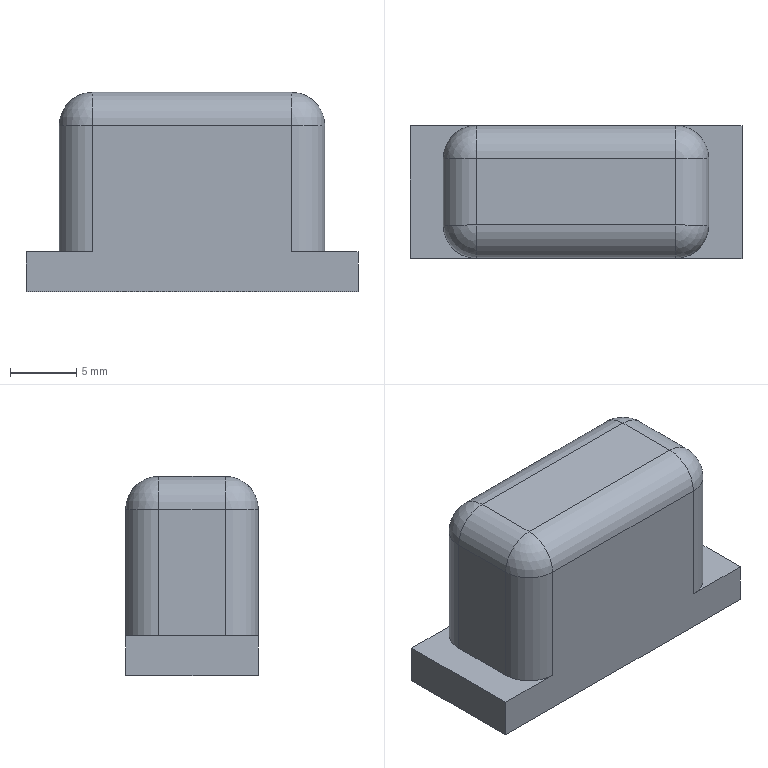NC program | NX | posted with a generic post | part box 25 x 10 x 15 mm
Whole program:
N10 G17 G21 G94 G90
(FLOOR_WALL_COPY , TOOL : D50)
N12 T01 M6
N14 G54
N16 G17 G0 G90 X-42.5 Y0. S4000 M3
N18 G43 Z30. H1
N20 Z5.666
N22 G94 G1 Z2.666 F1000.
N24 X-39.5
N26 X39.5
N28 X42.5
N30 Z5.666
N32 G0 Z30.
N34 X-42.5
N36 Z5.333
N38 G1 Z2.333
N40 X-39.5
N42 X39.5
N44 X42.5
N46 Z5.333
N48 G0 Z30.
N50 X-42.5
N52 Z5.
N54 G1 Z2.
N56 X-39.5
N58 X39.5
N60 X42.5
N62 Z5.
N64 G0 Z30.
N66 X-42.5
N68 Z4.667
N70 G1 Z1.667
N72 X-39.5
N74 X39.5
N76 X42.5
N78 Z4.667
N80 G0 Z30.
N82 X-42.5
N84 Z4.333
N86 G1 Z1.333
N88 X-39.5
N90 X39.5
N92 X42.5
N94 Z4.333
N96 G0 Z30.
N98 X-42.5
N100 Z4.
N102 G1 Z1.
N104 X-39.5
N106 X39.5
N108 X42.5
N110 Z4.
N112 G0 Z30.
N114 X-42.5
N116 Z3.667
N118 G1 Z0.667
N120 X-39.5
N122 X39.5
N124 X42.5
N126 Z3.667
N128 G0 Z30.
N130 X-42.5
N132 Z3.333
N134 G1 Z0.333
N136 X-39.5
N138 X39.5
N140 X42.5
N142 Z3.333
N144 G0 Z30.
N146 X-42.5
N148 Z3.
N150 G1 Z0.
N152 X-39.5
N154 X39.5
N156 X42.5
N158 Z3.
N160 G0 Z30.
N162 M5
(PLANAR_MILL , TOOL : D6A45)
N164 T07 M6
N166 G54
N168 G17 G0 G90 X1.27 Y-7.1 S8000 M3
N170 G43 Z30. H7
N172 Z0.5
N174 G94 G1 Z-1. F1250.
N176 X0.866 Y-6.4
N178 G3 X0. Y-5.9 R1.
N180 G1 X-12.4
N182 G2 X-13.4 Y-4.9 R1.
N184 G1 Y4.9
N186 G2 X-12.4 Y5.9 R1.
N188 G1 X12.4
N190 G2 X13.4 Y4.9 R1.
N192 G1 Y-4.9
N194 G2 X12.4 Y-5.9 R1.
N196 G1 X0.
N198 G3 X-0.866 Y-6.4 R1.
N200 G1 X-1.27 Y-7.1
N202 Z0.5
N204 G0 Z30.
N206 M5
N208 M2